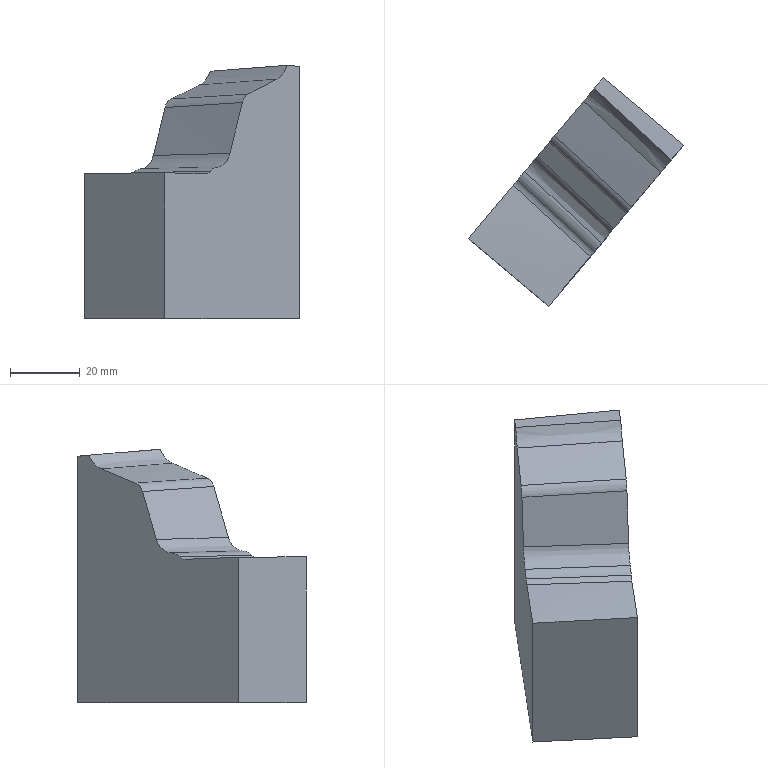Part | NX | features solid 2 | 1 solid | 14 faces | box 61.549 x 65.246 x 72.449 mm | volume 96298 mm3 | spline 9 | plane 5
STEP:
#1=CARTESIAN_POINT('',(566.959,407.194,-45.));
#2=VERTEX_POINT('',#1);
#3=CARTESIAN_POINT('',(566.959,407.194,25.462));
#4=VERTEX_POINT('',#3);
#5=CARTESIAN_POINT('',(566.959,407.194,-5.));
#6=DIRECTION('',(0.,0.,1.));
#7=VECTOR('',#6,1000.);
#8=LINE('',#5,#7);
#9=EDGE_CURVE('',#2,#4,#8,.T.);
#10=ORIENTED_EDGE('',*,*,#9,.T.);
#11=CARTESIAN_POINT('',(589.941,387.91,27.101));
#12=VERTEX_POINT('',#11);
#13=CARTESIAN_POINT('',(566.959,407.194,25.462));
#14=CARTESIAN_POINT('',(574.619,400.767,26.027));
#15=CARTESIAN_POINT('',(582.28,394.339,26.572));
#16=CARTESIAN_POINT('',(589.941,387.91,27.101));
#17=B_SPLINE_CURVE_WITH_KNOTS('',3,(#13,#14,#15,#16),.UNSPECIFIED.,.F.,.F.,(4,4),(0.,0.03004),.UNSPECIFIED.);
#18=EDGE_CURVE('',#4,#12,#17,.T.);
#19=ORIENTED_EDGE('',*,*,#18,.T.);
#20=CARTESIAN_POINT('',(589.941,387.91,-45.));
#21=VERTEX_POINT('',#20);
#22=CARTESIAN_POINT('',(589.941,387.91,-5.));
#23=DIRECTION('',(0.,0.,1.));
#24=VECTOR('',#23,1000.);
#25=LINE('',#22,#24);
#26=EDGE_CURVE('',#21,#12,#25,.T.);
#27=ORIENTED_EDGE('',*,*,#26,.F.);
#28=CARTESIAN_POINT('',(1441.684,-326.787,-45.));
#29=DIRECTION('',(-0.766,0.6428,0.));
#30=VECTOR('',#29,1000.);
#31=LINE('',#28,#30);
#32=EDGE_CURVE('',#2,#21,#31,.F.);
#33=ORIENTED_EDGE('',*,*,#32,.F.);
#34=EDGE_LOOP('',(#10,#19,#27,#33));
#35=FACE_BOUND('',#34,.T.);
#36=CARTESIAN_POINT('',(555.469,416.836,-5.));
#37=DIRECTION('',(0.6428,0.766,0.));
#38=DIRECTION('',(0.,0.,1.));
#39=AXIS2_PLACEMENT_3D('',#36,#37,#38);
#40=PLANE('',#39);
#41=ADVANCED_FACE('',(#35),#40,.T.);
#42=ORIENTED_EDGE('',*,*,#26,.T.);
#43=CARTESIAN_POINT('',(586.365,383.649,27.449));
#44=VERTEX_POINT('',#43);
#45=CARTESIAN_POINT('',(589.941,387.91,27.101));
#46=CARTESIAN_POINT('',(588.749,386.49,27.217));
#47=CARTESIAN_POINT('',(587.557,385.069,27.334));
#48=CARTESIAN_POINT('',(586.365,383.649,27.449));
#49=B_SPLINE_CURVE_WITH_KNOTS('',3,(#45,#46,#47,#48),.UNSPECIFIED.,.F.,.F.,(4,4),(0.,0.005573),.UNSPECIFIED.);
#50=EDGE_CURVE('',#12,#44,#49,.T.);
#51=ORIENTED_EDGE('',*,*,#50,.T.);
#52=CARTESIAN_POINT('',(583.395,380.11,23.455));
#53=VERTEX_POINT('',#52);
#54=CARTESIAN_POINT('',(586.365,383.649,27.449));
#55=CARTESIAN_POINT('',(585.756,382.923,25.561));
#56=CARTESIAN_POINT('',(584.683,381.644,24.119));
#57=CARTESIAN_POINT('',(583.394,380.108,23.454));
#58=B_SPLINE_CURVE_WITH_KNOTS('',3,(#54,#55,#56,#57),.UNSPECIFIED.,.F.,.F.,(4,4),(0.,0.006214),.UNSPECIFIED.);
#59=EDGE_CURVE('',#44,#53,#58,.T.);
#60=ORIENTED_EDGE('',*,*,#59,.T.);
#61=CARTESIAN_POINT('',(575.129,370.258,19.19));
#62=VERTEX_POINT('',#61);
#63=CARTESIAN_POINT('',(583.396,380.111,23.455));
#64=CARTESIAN_POINT('',(580.64,376.826,22.034));
#65=CARTESIAN_POINT('',(577.885,373.542,20.612));
#66=CARTESIAN_POINT('',(575.129,370.258,19.19));
#67=B_SPLINE_CURVE_WITH_KNOTS('',3,(#63,#64,#65,#66),.UNSPECIFIED.,.F.,.F.,(4,4),(0.0002168,0.01377),.UNSPECIFIED.);
#68=EDGE_CURVE('',#53,#62,#67,.T.);
#69=ORIENTED_EDGE('',*,*,#68,.T.);
#70=CARTESIAN_POINT('',(573.535,368.359,16.809));
#71=VERTEX_POINT('',#70);
#72=CARTESIAN_POINT('',(575.129,370.258,19.19));
#73=CARTESIAN_POINT('',(574.4,369.39,18.814));
#74=CARTESIAN_POINT('',(573.806,368.681,17.926));
#75=CARTESIAN_POINT('',(573.535,368.359,16.809));
#76=B_SPLINE_CURVE_WITH_KNOTS('',3,(#72,#73,#74,#75),.UNSPECIFIED.,.F.,.F.,(4,4),(0.,0.003553),.UNSPECIFIED.);
#77=EDGE_CURVE('',#62,#71,#76,.T.);
#78=ORIENTED_EDGE('',*,*,#77,.T.);
#79=CARTESIAN_POINT('',(570.007,364.154,2.246));
#80=VERTEX_POINT('',#79);
#81=CARTESIAN_POINT('',(570.007,364.154,2.246));
#82=CARTESIAN_POINT('',(571.183,365.556,7.1));
#83=CARTESIAN_POINT('',(572.359,366.957,11.954));
#84=CARTESIAN_POINT('',(573.535,368.359,16.809));
#85=B_SPLINE_CURVE_WITH_KNOTS('',3,(#81,#82,#83,#84),.UNSPECIFIED.,.F.,.F.,(4,4),(0.006324,0.02189),.UNSPECIFIED.);
#86=EDGE_CURVE('',#80,#71,#85,.T.);
#87=ORIENTED_EDGE('',*,*,#86,.F.);
#88=CARTESIAN_POINT('',(566.485,359.957,-1.636));
#89=VERTEX_POINT('',#88);
#90=CARTESIAN_POINT('',(570.007,364.154,2.246));
#91=CARTESIAN_POINT('',(569.464,363.507,0.004322));
#92=CARTESIAN_POINT('',(568.025,361.791,-1.579));
#93=CARTESIAN_POINT('',(566.485,359.957,-1.636));
#94=B_SPLINE_CURVE_WITH_KNOTS('',3,(#90,#91,#92,#93),.UNSPECIFIED.,.F.,.F.,(4,4),(0.,0.007083),.UNSPECIFIED.);
#95=EDGE_CURVE('',#80,#89,#94,.T.);
#96=ORIENTED_EDGE('',*,*,#95,.T.);
#97=CARTESIAN_POINT('',(564.485,357.574,-2.817));
#98=VERTEX_POINT('',#97);
#99=CARTESIAN_POINT('',(564.485,357.574,-2.817));
#100=CARTESIAN_POINT('',(565.044,358.239,-2.083));
#101=CARTESIAN_POINT('',(565.755,359.087,-1.664));
#102=CARTESIAN_POINT('',(566.485,359.957,-1.636));
#103=B_SPLINE_CURVE_WITH_KNOTS('',3,(#99,#100,#101,#102),.UNSPECIFIED.,.F.,.F.,(4,4),(0.000003197,0.003403),.UNSPECIFIED.);
#104=EDGE_CURVE('',#98,#89,#103,.T.);
#105=ORIENTED_EDGE('',*,*,#104,.F.);
#106=CARTESIAN_POINT('',(563.201,356.043,-3.525));
#107=VERTEX_POINT('',#106);
#108=CARTESIAN_POINT('',(563.201,356.043,-3.525));
#109=CARTESIAN_POINT('',(563.668,356.6,-3.539));
#110=CARTESIAN_POINT('',(564.129,357.148,-3.285));
#111=CARTESIAN_POINT('',(564.485,357.574,-2.817));
#112=B_SPLINE_CURVE_WITH_KNOTS('',3,(#108,#109,#110,#111),.UNSPECIFIED.,.F.,.F.,(4,4),(0.,0.00217),.UNSPECIFIED.);
#113=EDGE_CURVE('',#107,#98,#112,.T.);
#114=ORIENTED_EDGE('',*,*,#113,.F.);
#115=CARTESIAN_POINT('',(551.374,341.948,-3.282));
#116=VERTEX_POINT('',#115);
#117=CARTESIAN_POINT('',(551.374,341.948,-3.282));
#118=CARTESIAN_POINT('',(555.317,346.647,-3.326));
#119=CARTESIAN_POINT('',(559.259,351.345,-3.407));
#120=CARTESIAN_POINT('',(563.201,356.043,-3.525));
#121=B_SPLINE_CURVE_WITH_KNOTS('',3,(#117,#118,#119,#120),.UNSPECIFIED.,.F.,.F.,(4,4),(0.,0.0184),.UNSPECIFIED.);
#122=EDGE_CURVE('',#116,#107,#121,.T.);
#123=ORIENTED_EDGE('',*,*,#122,.F.);
#124=CARTESIAN_POINT('',(551.374,341.948,-45.));
#125=VERTEX_POINT('',#124);
#126=CARTESIAN_POINT('',(551.374,341.948,-5.));
#127=DIRECTION('',(0.,0.,-1.));
#128=VECTOR('',#127,1000.);
#129=LINE('',#126,#128);
#130=EDGE_CURVE('',#125,#116,#129,.F.);
#131=ORIENTED_EDGE('',*,*,#130,.F.);
#132=CARTESIAN_POINT('',(548.16,338.117,-45.));
#133=DIRECTION('',(-0.6428,-0.766,0.));
#134=VECTOR('',#133,1000.);
#135=LINE('',#132,#134);
#136=EDGE_CURVE('',#125,#21,#135,.F.);
#137=ORIENTED_EDGE('',*,*,#136,.T.);
#138=EDGE_LOOP('',(#42,#51,#60,#69,#78,#87,#96,#105,#114,#123,#131,#137));
#139=FACE_BOUND('',#138,.T.);
#140=CARTESIAN_POINT('',(548.16,338.117,-5.));
#141=DIRECTION('',(0.766,-0.6428,0.));
#142=DIRECTION('',(0.6428,0.766,0.));
#143=AXIS2_PLACEMENT_3D('',#140,#141,#142);
#144=PLANE('',#143);
#145=ADVANCED_FACE('',(#139),#144,.T.);
#146=CARTESIAN_POINT('',(564.326,404.056,25.737));
#147=VERTEX_POINT('',#146);
#148=CARTESIAN_POINT('',(566.959,407.194,25.462));
#149=CARTESIAN_POINT('',(566.082,406.148,25.554));
#150=CARTESIAN_POINT('',(565.204,405.102,25.646));
#151=CARTESIAN_POINT('',(564.326,404.056,25.737));
#152=B_SPLINE_CURVE_WITH_KNOTS('',3,(#148,#149,#150,#151),.UNSPECIFIED.,.F.,.F.,(4,4),(0.,0.004106),.UNSPECIFIED.);
#153=EDGE_CURVE('',#4,#147,#152,.T.);
#154=ORIENTED_EDGE('',*,*,#153,.F.);
#155=ORIENTED_EDGE('',*,*,#9,.F.);
#156=CARTESIAN_POINT('',(528.392,361.231,-45.));
#157=VERTEX_POINT('',#156);
#158=CARTESIAN_POINT('',(525.178,357.401,-45.));
#159=DIRECTION('',(-0.6428,-0.766,0.));
#160=VECTOR('',#159,1000.);
#161=LINE('',#158,#160);
#162=EDGE_CURVE('',#157,#2,#161,.F.);
#163=ORIENTED_EDGE('',*,*,#162,.F.);
#164=CARTESIAN_POINT('',(528.392,361.231,-3.433));
#165=VERTEX_POINT('',#164);
#166=CARTESIAN_POINT('',(528.392,361.231,-5.));
#167=DIRECTION('',(0.,0.,-1.));
#168=VECTOR('',#167,1000.);
#169=LINE('',#166,#168);
#170=EDGE_CURVE('',#157,#165,#169,.F.);
#171=ORIENTED_EDGE('',*,*,#170,.T.);
#172=CARTESIAN_POINT('',(541.163,376.451,-3.994));
#173=VERTEX_POINT('',#172);
#174=CARTESIAN_POINT('',(528.392,361.231,-3.433));
#175=CARTESIAN_POINT('',(532.65,366.305,-3.577));
#176=CARTESIAN_POINT('',(536.907,371.379,-3.764));
#177=CARTESIAN_POINT('',(541.163,376.451,-3.994));
#178=B_SPLINE_CURVE_WITH_KNOTS('',3,(#174,#175,#176,#177),.UNSPECIFIED.,.F.,.F.,(4,4),(0.,0.01988),.UNSPECIFIED.);
#179=EDGE_CURVE('',#165,#173,#178,.T.);
#180=ORIENTED_EDGE('',*,*,#179,.T.);
#181=CARTESIAN_POINT('',(542.453,377.988,-3.316));
#182=VERTEX_POINT('',#181);
#183=CARTESIAN_POINT('',(541.163,376.451,-3.994));
#184=CARTESIAN_POINT('',(541.63,377.007,-4.019));
#185=CARTESIAN_POINT('',(542.092,377.558,-3.777));
#186=CARTESIAN_POINT('',(542.453,377.988,-3.316));
#187=B_SPLINE_CURVE_WITH_KNOTS('',3,(#183,#184,#185,#186),.UNSPECIFIED.,.F.,.F.,(4,4),(0.,0.002169),.UNSPECIFIED.);
#188=EDGE_CURVE('',#173,#182,#187,.T.);
#189=ORIENTED_EDGE('',*,*,#188,.T.);
#190=CARTESIAN_POINT('',(544.495,380.422,-2.184));
#191=VERTEX_POINT('',#190);
#192=CARTESIAN_POINT('',(542.453,377.988,-3.316));
#193=CARTESIAN_POINT('',(543.027,378.672,-2.585));
#194=CARTESIAN_POINT('',(543.754,379.539,-2.182));
#195=CARTESIAN_POINT('',(544.495,380.422,-2.184));
#196=B_SPLINE_CURVE_WITH_KNOTS('',3,(#192,#193,#194,#195),.UNSPECIFIED.,.F.,.F.,(4,4),(0.000003374,0.003451),.UNSPECIFIED.);
#197=EDGE_CURVE('',#182,#191,#196,.T.);
#198=ORIENTED_EDGE('',*,*,#197,.T.);
#199=CARTESIAN_POINT('',(548.104,384.723,1.672));
#200=VERTEX_POINT('',#199);
#201=CARTESIAN_POINT('',(548.104,384.723,1.672));
#202=CARTESIAN_POINT('',(547.546,384.058,-0.6026));
#203=CARTESIAN_POINT('',(546.061,382.288,-2.188));
#204=CARTESIAN_POINT('',(544.495,380.422,-2.184));
#205=B_SPLINE_CURVE_WITH_KNOTS('',3,(#201,#202,#203,#204),.UNSPECIFIED.,.F.,.F.,(4,4),(0.,0.007202),.UNSPECIFIED.);
#206=EDGE_CURVE('',#200,#191,#205,.T.);
#207=ORIENTED_EDGE('',*,*,#206,.F.);
#208=CARTESIAN_POINT('',(551.467,388.73,15.371));
#209=VERTEX_POINT('',#208);
#210=CARTESIAN_POINT('',(548.104,384.723,1.672));
#211=CARTESIAN_POINT('',(549.225,386.059,6.238));
#212=CARTESIAN_POINT('',(550.346,387.395,10.805));
#213=CARTESIAN_POINT('',(551.467,388.73,15.371));
#214=B_SPLINE_CURVE_WITH_KNOTS('',3,(#210,#211,#212,#213),.UNSPECIFIED.,.F.,.F.,(4,4),(0.006972,0.02164),.UNSPECIFIED.);
#215=EDGE_CURVE('',#200,#209,#214,.T.);
#216=ORIENTED_EDGE('',*,*,#215,.T.);
#217=CARTESIAN_POINT('',(553.09,390.665,17.754));
#218=VERTEX_POINT('',#217);
#219=CARTESIAN_POINT('',(553.09,390.665,17.754));
#220=CARTESIAN_POINT('',(552.35,389.783,17.39));
#221=CARTESIAN_POINT('',(551.743,389.06,16.499));
#222=CARTESIAN_POINT('',(551.467,388.73,15.371));
#223=B_SPLINE_CURVE_WITH_KNOTS('',3,(#219,#220,#221,#222),.UNSPECIFIED.,.F.,.F.,(4,4),(0.,0.003592),.UNSPECIFIED.);
#224=EDGE_CURVE('',#218,#209,#223,.T.);
#225=ORIENTED_EDGE('',*,*,#224,.F.);
#226=CARTESIAN_POINT('',(561.322,400.475,21.808));
#227=VERTEX_POINT('',#226);
#228=CARTESIAN_POINT('',(561.323,400.476,21.808));
#229=CARTESIAN_POINT('',(558.578,397.206,20.457));
#230=CARTESIAN_POINT('',(555.834,393.935,19.106));
#231=CARTESIAN_POINT('',(553.09,390.665,17.754));
#232=B_SPLINE_CURVE_WITH_KNOTS('',3,(#228,#229,#230,#231),.UNSPECIFIED.,.F.,.F.,(4,4),(0.0001803,0.01361),.UNSPECIFIED.);
#233=EDGE_CURVE('',#227,#218,#232,.T.);
#234=ORIENTED_EDGE('',*,*,#233,.F.);
#235=CARTESIAN_POINT('',(564.326,404.056,25.737));
#236=CARTESIAN_POINT('',(563.7,403.31,23.864));
#237=CARTESIAN_POINT('',(562.615,402.017,22.445));
#238=CARTESIAN_POINT('',(561.322,400.475,21.808));
#239=B_SPLINE_CURVE_WITH_KNOTS('',3,(#235,#236,#237,#238),.UNSPECIFIED.,.F.,.F.,(4,4),(0.,0.006211),.UNSPECIFIED.);
#240=EDGE_CURVE('',#147,#227,#239,.T.);
#241=ORIENTED_EDGE('',*,*,#240,.F.);
#242=EDGE_LOOP('',(#154,#155,#163,#171,#180,#189,#198,#207,#216,#225,#234,#241));
#243=FACE_BOUND('',#242,.T.);
#244=CARTESIAN_POINT('',(525.178,357.401,-5.));
#245=DIRECTION('',(0.766,-0.6428,0.));
#246=DIRECTION('',(0.6428,0.766,0.));
#247=AXIS2_PLACEMENT_3D('',#244,#245,#246);
#248=PLANE('',#247);
#249=ADVANCED_FACE('',(#243),#248,.F.);
#250=ORIENTED_EDGE('',*,*,#130,.T.);
#251=CARTESIAN_POINT('',(528.392,361.231,-3.433));
#252=CARTESIAN_POINT('',(536.052,354.803,-3.328));
#253=CARTESIAN_POINT('',(543.713,348.376,-3.277));
#254=CARTESIAN_POINT('',(551.374,341.948,-3.282));
#255=B_SPLINE_CURVE_WITH_KNOTS('',3,(#251,#252,#253,#254),.UNSPECIFIED.,.F.,.F.,(4,4),(0.,0.03),.UNSPECIFIED.);
#256=EDGE_CURVE('',#165,#116,#255,.T.);
#257=ORIENTED_EDGE('',*,*,#256,.F.);
#258=ORIENTED_EDGE('',*,*,#170,.F.);
#259=CARTESIAN_POINT('',(516.902,370.873,-45.));
#260=DIRECTION('',(0.766,-0.6428,0.));
#261=VECTOR('',#260,1000.);
#262=LINE('',#259,#261);
#263=EDGE_CURVE('',#157,#125,#262,.T.);
#264=ORIENTED_EDGE('',*,*,#263,.T.);
#265=EDGE_LOOP('',(#250,#257,#258,#264));
#266=FACE_BOUND('',#265,.T.);
#267=CARTESIAN_POINT('',(516.902,370.873,-5.));
#268=DIRECTION('',(0.6428,0.766,0.));
#269=DIRECTION('',(0.,0.,1.));
#270=AXIS2_PLACEMENT_3D('',#267,#268,#269);
#271=PLANE('',#270);
#272=ADVANCED_FACE('',(#266),#271,.F.);
#273=ORIENTED_EDGE('',*,*,#263,.F.);
#274=ORIENTED_EDGE('',*,*,#162,.T.);
#275=ORIENTED_EDGE('',*,*,#32,.T.);
#276=ORIENTED_EDGE('',*,*,#136,.F.);
#277=EDGE_LOOP('',(#273,#274,#275,#276));
#278=FACE_BOUND('',#277,.T.);
#279=CARTESIAN_POINT('',(1076.581,-761.9,-45.));
#280=DIRECTION('',(0.,0.,1.));
#281=DIRECTION('',(1.,0.,0.));
#282=AXIS2_PLACEMENT_3D('',#279,#280,#281);
#283=PLANE('',#282);
#284=ADVANCED_FACE('',(#278),#283,.F.);
#285=CARTESIAN_POINT('',(541.163,376.451,-3.994));
#286=CARTESIAN_POINT('',(548.532,369.705,-3.778));
#287=CARTESIAN_POINT('',(555.864,362.916,-3.62));
#288=CARTESIAN_POINT('',(563.201,356.043,-3.525));
#289=B_SPLINE_CURVE_WITH_KNOTS('',3,(#285,#286,#287,#288),.UNSPECIFIED.,.F.,.F.,(4,4),(0.5481,0.8366),.UNSPECIFIED.);
#290=EDGE_CURVE('',#173,#107,#289,.T.);
#291=ORIENTED_EDGE('',*,*,#290,.T.);
#292=ORIENTED_EDGE('',*,*,#113,.T.);
#293=CARTESIAN_POINT('',(564.485,357.574,-2.817));
#294=CARTESIAN_POINT('',(557.239,364.365,-2.921));
#295=CARTESIAN_POINT('',(549.881,371.184,-3.088));
#296=CARTESIAN_POINT('',(542.453,377.988,-3.316));
#297=B_SPLINE_CURVE_WITH_KNOTS('',3,(#293,#294,#295,#296),.UNSPECIFIED.,.F.,.F.,(4,4),(0.1708,0.4613),.UNSPECIFIED.);
#298=EDGE_CURVE('',#98,#182,#297,.T.);
#299=ORIENTED_EDGE('',*,*,#298,.T.);
#300=ORIENTED_EDGE('',*,*,#188,.F.);
#301=EDGE_LOOP('',(#291,#292,#299,#300));
#302=FACE_BOUND('',#301,.T.);
#303=CARTESIAN_POINT('',(540.974,376.624,-4.));
#304=CARTESIAN_POINT('',(541.267,376.942,-4.014));
#305=CARTESIAN_POINT('',(541.56,377.264,-3.951));
#306=CARTESIAN_POINT('',(541.841,377.575,-3.809));
#307=CARTESIAN_POINT('',(542.097,377.861,-3.595));
#308=CARTESIAN_POINT('',(542.319,378.111,-3.321));
#309=CARTESIAN_POINT('',(541.45,376.188,-3.986));
#310=CARTESIAN_POINT('',(541.743,376.506,-4.));
#311=CARTESIAN_POINT('',(542.036,376.828,-3.937));
#312=CARTESIAN_POINT('',(542.317,377.138,-3.795));
#313=CARTESIAN_POINT('',(542.574,377.424,-3.58));
#314=CARTESIAN_POINT('',(542.795,377.675,-3.306));
#315=CARTESIAN_POINT('',(541.926,375.752,-3.972));
#316=CARTESIAN_POINT('',(542.219,376.07,-3.986));
#317=CARTESIAN_POINT('',(542.513,376.392,-3.923));
#318=CARTESIAN_POINT('',(542.794,376.702,-3.781));
#319=CARTESIAN_POINT('',(543.05,376.988,-3.566));
#320=CARTESIAN_POINT('',(543.272,377.238,-3.291));
#321=CARTESIAN_POINT('',(542.403,375.316,-3.958));
#322=CARTESIAN_POINT('',(542.696,375.634,-3.973));
#323=CARTESIAN_POINT('',(542.989,375.955,-3.909));
#324=CARTESIAN_POINT('',(543.27,376.265,-3.766));
#325=CARTESIAN_POINT('',(543.527,376.551,-3.552));
#326=CARTESIAN_POINT('',(543.749,376.801,-3.277));
#327=CARTESIAN_POINT('',(545.037,372.9,-3.884));
#328=CARTESIAN_POINT('',(545.33,373.218,-3.898));
#329=CARTESIAN_POINT('',(545.624,373.539,-3.833));
#330=CARTESIAN_POINT('',(545.906,373.849,-3.69));
#331=CARTESIAN_POINT('',(546.162,374.133,-3.475));
#332=CARTESIAN_POINT('',(546.385,374.382,-3.199));
#333=CARTESIAN_POINT('',(547.66,370.487,-3.816));
#334=CARTESIAN_POINT('',(547.954,370.804,-3.829));
#335=CARTESIAN_POINT('',(548.248,371.124,-3.764));
#336=CARTESIAN_POINT('',(548.53,371.433,-3.62));
#337=CARTESIAN_POINT('',(548.787,371.717,-3.404));
#338=CARTESIAN_POINT('',(549.01,371.965,-3.128));
#339=CARTESIAN_POINT('',(549.8,368.512,-3.765));
#340=CARTESIAN_POINT('',(550.094,368.83,-3.777));
#341=CARTESIAN_POINT('',(550.388,369.149,-3.711));
#342=CARTESIAN_POINT('',(550.671,369.458,-3.567));
#343=CARTESIAN_POINT('',(550.928,369.741,-3.35));
#344=CARTESIAN_POINT('',(551.151,369.988,-3.074));
#345=CARTESIAN_POINT('',(552.884,365.659,-3.698));
#346=CARTESIAN_POINT('',(553.178,365.976,-3.709));
#347=CARTESIAN_POINT('',(553.473,366.295,-3.642));
#348=CARTESIAN_POINT('',(553.756,366.603,-3.497));
#349=CARTESIAN_POINT('',(554.014,366.885,-3.279));
#350=CARTESIAN_POINT('',(554.237,367.131,-3.002));
#351=CARTESIAN_POINT('',(555.953,362.809,-3.639));
#352=CARTESIAN_POINT('',(556.248,363.125,-3.65));
#353=CARTESIAN_POINT('',(556.543,363.443,-3.582));
#354=CARTESIAN_POINT('',(556.826,363.75,-3.436));
#355=CARTESIAN_POINT('',(557.085,364.031,-3.217));
#356=CARTESIAN_POINT('',(557.308,364.276,-2.939));
#357=CARTESIAN_POINT('',(556.896,361.931,-3.622));
#358=CARTESIAN_POINT('',(557.191,362.248,-3.632));
#359=CARTESIAN_POINT('',(557.486,362.566,-3.564));
#360=CARTESIAN_POINT('',(557.77,362.872,-3.418));
#361=CARTESIAN_POINT('',(558.028,363.153,-3.199));
#362=CARTESIAN_POINT('',(558.252,363.398,-2.921));
#363=CARTESIAN_POINT('',(558.752,360.203,-3.59));
#364=CARTESIAN_POINT('',(559.048,360.519,-3.599));
#365=CARTESIAN_POINT('',(559.344,360.836,-3.531));
#366=CARTESIAN_POINT('',(559.627,361.142,-3.384));
#367=CARTESIAN_POINT('',(559.886,361.423,-3.165));
#368=CARTESIAN_POINT('',(560.109,361.667,-2.886));
#369=CARTESIAN_POINT('',(560.603,358.475,-3.561));
#370=CARTESIAN_POINT('',(560.899,358.79,-3.57));
#371=CARTESIAN_POINT('',(561.195,359.108,-3.501));
#372=CARTESIAN_POINT('',(561.479,359.413,-3.353));
#373=CARTESIAN_POINT('',(561.738,359.693,-3.134));
#374=CARTESIAN_POINT('',(561.962,359.936,-2.855));
#375=CARTESIAN_POINT('',(561.514,357.623,-3.548));
#376=CARTESIAN_POINT('',(561.81,357.939,-3.557));
#377=CARTESIAN_POINT('',(562.107,358.256,-3.487));
#378=CARTESIAN_POINT('',(562.391,358.561,-3.339));
#379=CARTESIAN_POINT('',(562.65,358.84,-3.12));
#380=CARTESIAN_POINT('',(562.874,359.084,-2.84));
#381=CARTESIAN_POINT('',(562.424,356.772,-3.535));
#382=CARTESIAN_POINT('',(562.72,357.087,-3.544));
#383=CARTESIAN_POINT('',(563.017,357.404,-3.474));
#384=CARTESIAN_POINT('',(563.301,357.709,-3.326));
#385=CARTESIAN_POINT('',(563.56,357.988,-3.106));
#386=CARTESIAN_POINT('',(563.784,358.231,-2.827));
#387=CARTESIAN_POINT('',(563.332,355.921,-3.524));
#388=CARTESIAN_POINT('',(563.629,356.236,-3.532));
#389=CARTESIAN_POINT('',(563.925,356.553,-3.462));
#390=CARTESIAN_POINT('',(564.21,356.858,-3.313));
#391=CARTESIAN_POINT('',(564.469,357.136,-3.093));
#392=CARTESIAN_POINT('',(564.693,357.379,-2.814));
#393=B_SPLINE_SURFACE_WITH_KNOTS('',5,5,((#303,#304,#305,#306,#307,#308),(#309,#310,#311,#312,#313,#314),(#315,#316,#317,#318,#319,#320),(#321,#322,#323,#324,#325,#326),(#327,#328,#329,#330,#331,#332),(#333,#334,#335,#336,#337,#338),(#339,#340,#341,#342,#343,#344),(#345,#346,#347,#348,#349,#350),(#351,#352,#353,#354,#355,#356),(#357,#358,#359,#360,#361,#362),(#363,#364,#365,#366,#367,#368),(#369,#370,#371,#372,#373,#374),(#375,#376,#377,#378,#379,#380),(#381,#382,#383,#384,#385,#386),(#387,#388,#389,#390,#391,#392)),.UNSPECIFIED.,.F.,.F.,.F.,(6,3,3,3,6),(6,6),(0.537,0.568,0.7087,0.7712,0.832),(0.,1.),.UNSPECIFIED.);
#394=ADVANCED_FACE('',(#302),#393,.T.);
#395=ORIENTED_EDGE('',*,*,#298,.F.);
#396=ORIENTED_EDGE('',*,*,#104,.T.);
#397=CARTESIAN_POINT('',(566.485,359.957,-1.636));
#398=CARTESIAN_POINT('',(564.733,361.609,-1.666));
#399=CARTESIAN_POINT('',(562.019,364.16,-1.716));
#400=CARTESIAN_POINT('',(558.279,367.657,-1.798));
#401=CARTESIAN_POINT('',(556.002,369.779,-1.852));
#402=CARTESIAN_POINT('',(554.201,371.454,-1.898));
#403=CARTESIAN_POINT('',(552.911,372.652,-1.932));
#404=CARTESIAN_POINT('',(551.301,374.145,-1.976));
#405=CARTESIAN_POINT('',(549.875,375.465,-2.017));
#406=CARTESIAN_POINT('',(548.553,376.686,-2.056));
#407=CARTESIAN_POINT('',(546.747,378.351,-2.111));
#408=CARTESIAN_POINT('',(545.398,379.593,-2.154));
#409=CARTESIAN_POINT('',(544.495,380.422,-2.184));
#410=B_SPLINE_CURVE_WITH_KNOTS('',3,(#397,#398,#399,#400,#401,#402,#403,#404,#405,#406,#407,#408,#409),.UNSPECIFIED.,.F.,.F.,(4,1,1,1,1,1,1,1,1,1,4),(0.1737,0.2446,0.2801,0.3156,0.3334,0.3511,0.3689,0.3866,0.4044,0.4221,0.4576),.UNSPECIFIED.);
#411=EDGE_CURVE('',#89,#191,#410,.T.);
#412=ORIENTED_EDGE('',*,*,#411,.T.);
#413=ORIENTED_EDGE('',*,*,#197,.F.);
#414=EDGE_LOOP('',(#395,#396,#412,#413));
#415=FACE_BOUND('',#414,.T.);
#416=CARTESIAN_POINT('',(566.77,359.779,-1.631));
#417=CARTESIAN_POINT('',(566.299,359.273,-1.639));
#418=CARTESIAN_POINT('',(565.829,358.768,-1.767));
#419=CARTESIAN_POINT('',(565.38,358.283,-2.014));
#420=CARTESIAN_POINT('',(564.971,357.838,-2.37));
#421=CARTESIAN_POINT('',(564.615,357.449,-2.817));
#422=CARTESIAN_POINT('',(565.115,361.333,-1.659));
#423=CARTESIAN_POINT('',(564.643,360.827,-1.666));
#424=CARTESIAN_POINT('',(564.174,360.321,-1.793));
#425=CARTESIAN_POINT('',(563.725,359.835,-2.039));
#426=CARTESIAN_POINT('',(563.316,359.39,-2.394));
#427=CARTESIAN_POINT('',(562.961,358.999,-2.841));
#428=CARTESIAN_POINT('',(563.454,362.887,-1.689));
#429=CARTESIAN_POINT('',(562.984,362.381,-1.695));
#430=CARTESIAN_POINT('',(562.515,361.875,-1.821));
#431=CARTESIAN_POINT('',(562.067,361.388,-2.067));
#432=CARTESIAN_POINT('',(561.658,360.942,-2.421));
#433=CARTESIAN_POINT('',(561.302,360.551,-2.867));
#434=CARTESIAN_POINT('',(561.79,364.442,-1.721));
#435=CARTESIAN_POINT('',(561.32,363.936,-1.727));
#436=CARTESIAN_POINT('',(560.851,363.429,-1.852));
#437=CARTESIAN_POINT('',(560.404,362.942,-2.097));
#438=CARTESIAN_POINT('',(559.995,362.494,-2.451));
#439=CARTESIAN_POINT('',(559.64,362.102,-2.896));
#440=CARTESIAN_POINT('',(557.337,368.595,-1.816));
#441=CARTESIAN_POINT('',(556.868,368.087,-1.82));
#442=CARTESIAN_POINT('',(556.4,367.579,-1.943));
#443=CARTESIAN_POINT('',(555.954,367.089,-2.185));
#444=CARTESIAN_POINT('',(555.546,366.639,-2.537));
#445=CARTESIAN_POINT('',(555.192,366.245,-2.981));
#446=CARTESIAN_POINT('',(552.853,372.751,-1.93));
#447=CARTESIAN_POINT('',(552.385,372.242,-1.931));
#448=CARTESIAN_POINT('',(551.919,371.732,-2.052));
#449=CARTESIAN_POINT('',(551.473,371.241,-2.293));
#450=CARTESIAN_POINT('',(551.066,370.789,-2.643));
#451=CARTESIAN_POINT('',(550.713,370.392,-3.085));
#452=CARTESIAN_POINT('',(550.038,375.351,-2.008));
#453=CARTESIAN_POINT('',(549.571,374.842,-2.009));
#454=CARTESIAN_POINT('',(549.105,374.331,-2.128));
#455=CARTESIAN_POINT('',(548.66,373.838,-2.368));
#456=CARTESIAN_POINT('',(548.254,373.385,-2.717));
#457=CARTESIAN_POINT('',(547.901,372.986,-3.158));
#458=CARTESIAN_POINT('',(547.211,377.953,-2.095));
#459=CARTESIAN_POINT('',(546.744,377.443,-2.094));
#460=CARTESIAN_POINT('',(546.279,376.931,-2.212));
#461=CARTESIAN_POINT('',(545.835,376.437,-2.45));
#462=CARTESIAN_POINT('',(545.429,375.982,-2.798));
#463=CARTESIAN_POINT('',(545.076,375.582,-3.238));
#464=CARTESIAN_POINT('',(544.371,380.557,-2.189));
#465=CARTESIAN_POINT('',(543.905,380.046,-2.186));
#466=CARTESIAN_POINT('',(543.441,379.533,-2.303));
#467=CARTESIAN_POINT('',(542.997,379.038,-2.54));
#468=CARTESIAN_POINT('',(542.592,378.582,-2.886));
#469=CARTESIAN_POINT('',(542.24,378.18,-3.325));
#470=B_SPLINE_SURFACE_WITH_KNOTS('',5,5,((#416,#417,#418,#419,#420,#421),(#422,#423,#424,#425,#426,#427),(#428,#429,#430,#431,#432,#433),(#434,#435,#436,#437,#438,#439),(#440,#441,#442,#443,#444,#445),(#446,#447,#448,#449,#450,#451),(#452,#453,#454,#455,#456,#457),(#458,#459,#460,#461,#462,#463),(#464,#465,#466,#467,#468,#469)),.UNSPECIFIED.,.F.,.F.,.F.,(6,3,6),(6,6),(0.1683,0.2783,0.4618),(0.,1.),.UNSPECIFIED.);
#471=ADVANCED_FACE('',(#415),#470,.T.);
#472=ORIENTED_EDGE('',*,*,#206,.T.);
#473=ORIENTED_EDGE('',*,*,#411,.F.);
#474=ORIENTED_EDGE('',*,*,#95,.F.);
#475=CARTESIAN_POINT('',(548.104,384.723,1.672));
#476=CARTESIAN_POINT('',(555.53,377.849,1.927));
#477=CARTESIAN_POINT('',(562.819,371.001,2.118));
#478=CARTESIAN_POINT('',(570.007,364.154,2.246));
#479=B_SPLINE_CURVE_WITH_KNOTS('',3,(#475,#476,#477,#478),.UNSPECIFIED.,.F.,.F.,(4,4),(0.5365,0.8266),.UNSPECIFIED.);
#480=EDGE_CURVE('',#200,#80,#479,.T.);
#481=ORIENTED_EDGE('',*,*,#480,.F.);
#482=EDGE_LOOP('',(#472,#473,#474,#481));
#483=FACE_BOUND('',#482,.T.);
#484=CARTESIAN_POINT('',(566.616,359.834,-1.634));
#485=CARTESIAN_POINT('',(567.598,360.864,-1.599));
#486=CARTESIAN_POINT('',(568.569,361.89,-1.141));
#487=CARTESIAN_POINT('',(569.413,362.79,-0.2641));
#488=CARTESIAN_POINT('',(570.021,363.448,0.9195));
#489=CARTESIAN_POINT('',(570.356,363.821,2.252));
#490=CARTESIAN_POINT('',(566.277,360.154,-1.64));
#491=CARTESIAN_POINT('',(567.259,361.185,-1.605));
#492=CARTESIAN_POINT('',(568.23,362.211,-1.148));
#493=CARTESIAN_POINT('',(569.074,363.112,-0.2707));
#494=CARTESIAN_POINT('',(569.682,363.771,0.9132));
#495=CARTESIAN_POINT('',(570.016,364.145,2.246));
#496=CARTESIAN_POINT('',(565.937,360.474,-1.646));
#497=CARTESIAN_POINT('',(566.919,361.505,-1.611));
#498=CARTESIAN_POINT('',(567.89,362.533,-1.155));
#499=CARTESIAN_POINT('',(568.734,363.434,-0.2774));
#500=CARTESIAN_POINT('',(569.343,364.094,0.9067));
#501=CARTESIAN_POINT('',(569.677,364.468,2.24));
#502=CARTESIAN_POINT('',(565.597,360.794,-1.651));
#503=CARTESIAN_POINT('',(566.579,361.826,-1.618));
#504=CARTESIAN_POINT('',(567.55,362.854,-1.161));
#505=CARTESIAN_POINT('',(568.395,363.757,-0.2843));
#506=CARTESIAN_POINT('',(569.003,364.417,0.9002));
#507=CARTESIAN_POINT('',(569.337,364.791,2.234));
#508=CARTESIAN_POINT('',(564.816,361.53,-1.665));
#509=CARTESIAN_POINT('',(565.798,362.563,-1.633));
#510=CARTESIAN_POINT('',(566.77,363.593,-1.177));
#511=CARTESIAN_POINT('',(567.614,364.497,-0.3002));
#512=CARTESIAN_POINT('',(568.223,365.159,0.8848));
#513=CARTESIAN_POINT('',(568.557,365.534,2.219));
#514=CARTESIAN_POINT('',(564.033,362.266,-1.679));
#515=CARTESIAN_POINT('',(565.016,363.3,-1.649));
#516=CARTESIAN_POINT('',(565.988,364.331,-1.194));
#517=CARTESIAN_POINT('',(566.833,365.237,-0.3168));
#518=CARTESIAN_POINT('',(567.441,365.9,0.8689));
#519=CARTESIAN_POINT('',(567.775,366.277,2.204));
#520=CARTESIAN_POINT('',(563.591,362.681,-1.688));
#521=CARTESIAN_POINT('',(564.574,363.716,-1.658));
#522=CARTESIAN_POINT('',(565.546,364.748,-1.203));
#523=CARTESIAN_POINT('',(566.391,365.655,-0.3263));
#524=CARTESIAN_POINT('',(567.,366.319,0.8597));
#525=CARTESIAN_POINT('',(567.333,366.697,2.195));
#526=CARTESIAN_POINT('',(561.036,365.081,-1.736));
#527=CARTESIAN_POINT('',(562.019,366.12,-1.711));
#528=CARTESIAN_POINT('',(562.992,367.157,-1.259));
#529=CARTESIAN_POINT('',(563.838,368.07,-0.3824));
#530=CARTESIAN_POINT('',(564.447,368.739,0.8054));
#531=CARTESIAN_POINT('',(564.78,369.12,2.144));
#532=CARTESIAN_POINT('',(558.471,367.481,-1.792));
#533=CARTESIAN_POINT('',(559.454,368.524,-1.771));
#534=CARTESIAN_POINT('',(560.428,369.567,-1.322));
#535=CARTESIAN_POINT('',(561.275,370.485,-0.4448));
#536=CARTESIAN_POINT('',(561.884,371.159,0.7448));
#537=CARTESIAN_POINT('',(562.216,371.543,2.086));
#538=CARTESIAN_POINT('',(556.342,369.466,-1.842));
#539=CARTESIAN_POINT('',(557.326,370.512,-1.824));
#540=CARTESIAN_POINT('',(558.301,371.559,-1.377));
#541=CARTESIAN_POINT('',(559.148,372.482,-0.5006));
#542=CARTESIAN_POINT('',(559.757,373.16,0.6902));
#543=CARTESIAN_POINT('',(560.088,373.546,2.033));
#544=CARTESIAN_POINT('',(552.658,372.891,-1.936));
#545=CARTESIAN_POINT('',(553.643,373.943,-1.924));
#546=CARTESIAN_POINT('',(554.618,374.997,-1.481));
#547=CARTESIAN_POINT('',(555.466,375.928,-0.6044));
#548=CARTESIAN_POINT('',(556.074,376.612,0.5886));
#549=CARTESIAN_POINT('',(556.404,377.003,1.935));
#550=CARTESIAN_POINT('',(548.953,376.318,-2.043));
#551=CARTESIAN_POINT('',(549.938,377.374,-2.037));
#552=CARTESIAN_POINT('',(550.914,378.436,-1.597));
#553=CARTESIAN_POINT('',(551.762,379.374,-0.7209));
#554=CARTESIAN_POINT('',(552.37,380.065,0.4741));
#555=CARTESIAN_POINT('',(552.698,380.46,1.823));
#556=CARTESIAN_POINT('',(547.377,377.772,-2.091));
#557=CARTESIAN_POINT('',(548.362,378.83,-2.087));
#558=CARTESIAN_POINT('',(549.338,379.895,-1.648));
#559=CARTESIAN_POINT('',(550.186,380.836,-0.7726));
#560=CARTESIAN_POINT('',(550.794,381.529,0.4232));
#561=CARTESIAN_POINT('',(551.121,381.927,1.774));
#562=CARTESIAN_POINT('',(545.8,379.224,-2.141));
#563=CARTESIAN_POINT('',(546.784,380.284,-2.139));
#564=CARTESIAN_POINT('',(547.761,381.352,-1.702));
#565=CARTESIAN_POINT('',(548.609,382.296,-0.8265));
#566=CARTESIAN_POINT('',(549.216,382.992,0.37));
#567=CARTESIAN_POINT('',(549.544,383.391,1.722));
#568=CARTESIAN_POINT('',(544.224,380.671,-2.193));
#569=CARTESIAN_POINT('',(545.209,381.734,-2.194));
#570=CARTESIAN_POINT('',(546.185,382.804,-1.758));
#571=CARTESIAN_POINT('',(547.034,383.751,-0.8824));
#572=CARTESIAN_POINT('',(547.64,384.449,0.3147));
#573=CARTESIAN_POINT('',(547.967,384.851,1.668));
#574=B_SPLINE_SURFACE_WITH_KNOTS('',5,5,((#484,#485,#486,#487,#488,#489),(#490,#491,#492,#493,#494,#495),(#496,#497,#498,#499,#500,#501),(#502,#503,#504,#505,#506,#507),(#508,#509,#510,#511,#512,#513),(#514,#515,#516,#517,#518,#519),(#520,#521,#522,#523,#524,#525),(#526,#527,#528,#529,#530,#531),(#532,#533,#534,#535,#536,#537),(#538,#539,#540,#541,#542,#543),(#544,#545,#546,#547,#548,#549),(#550,#551,#552,#553,#554,#555),(#556,#557,#558,#559,#560,#561),(#562,#563,#564,#565,#566,#567),(#568,#569,#570,#571,#572,#573)),.UNSPECIFIED.,.F.,.F.,.F.,(6,3,3,3,6),(6,6),(0.1687,0.1915,0.2211,0.3626,0.4653),(0.,1.),.UNSPECIFIED.);
#575=ADVANCED_FACE('',(#483),#574,.F.);
#576=ORIENTED_EDGE('',*,*,#480,.T.);
#577=ORIENTED_EDGE('',*,*,#86,.T.);
#578=CARTESIAN_POINT('',(573.535,368.359,16.809));
#579=CARTESIAN_POINT('',(569.804,371.843,16.575));
#580=CARTESIAN_POINT('',(562.506,378.617,16.108));
#581=CARTESIAN_POINT('',(555.151,385.368,15.62));
#582=CARTESIAN_POINT('',(551.467,388.73,15.371));
#583=B_SPLINE_CURVE_WITH_KNOTS('',3,(#578,#579,#580,#581,#582),.UNSPECIFIED.,.F.,.F.,(4,1,4),(0.2733,0.3375,0.4017),.UNSPECIFIED.);
#584=EDGE_CURVE('',#71,#209,#583,.T.);
#585=ORIENTED_EDGE('',*,*,#584,.T.);
#586=ORIENTED_EDGE('',*,*,#215,.F.);
#587=EDGE_LOOP('',(#576,#577,#585,#586));
#588=FACE_BOUND('',#587,.T.);
#589=CARTESIAN_POINT('',(547.815,384.63,0.9737));
#590=CARTESIAN_POINT('',(551.117,389.22,15.672));
#591=CARTESIAN_POINT('',(552.344,380.488,1.225));
#592=CARTESIAN_POINT('',(555.654,385.054,15.929));
#593=CARTESIAN_POINT('',(556.862,376.334,1.47));
#594=CARTESIAN_POINT('',(560.18,380.875,16.18));
#595=CARTESIAN_POINT('',(561.369,372.166,1.711));
#596=CARTESIAN_POINT('',(564.695,376.683,16.426));
#597=CARTESIAN_POINT('',(565.863,367.985,1.946));
#598=CARTESIAN_POINT('',(569.197,372.478,16.668));
#599=CARTESIAN_POINT('',(570.346,363.791,2.177));
#600=CARTESIAN_POINT('',(573.688,368.26,16.903));
#601=B_SPLINE_SURFACE_WITH_KNOTS('',5,1,((#589,#590),(#591,#592),(#593,#594),(#595,#596),(#597,#598),(#599,#600)),.RULED_SURF.,.F.,.F.,.F.,(6,6),(2,2),(0.4854,0.5749),(0.3297,0.6804),.PIECEWISE_BEZIER_KNOTS.);
#602=ADVANCED_FACE('',(#588),#601,.T.);
#603=ORIENTED_EDGE('',*,*,#224,.T.);
#604=ORIENTED_EDGE('',*,*,#584,.F.);
#605=ORIENTED_EDGE('',*,*,#77,.F.);
#606=CARTESIAN_POINT('',(553.09,390.665,17.754));
#607=CARTESIAN_POINT('',(560.473,383.906,18.253));
#608=CARTESIAN_POINT('',(567.819,377.103,18.732));
#609=CARTESIAN_POINT('',(575.129,370.258,19.19));
#610=B_SPLINE_CURVE_WITH_KNOTS('',3,(#606,#607,#608,#609),.UNSPECIFIED.,.F.,.F.,(4,4),(0.593,0.7221),.UNSPECIFIED.);
#611=EDGE_CURVE('',#218,#62,#610,.T.);
#612=ORIENTED_EDGE('',*,*,#611,.F.);
#613=EDGE_LOOP('',(#603,#604,#605,#612));
#614=FACE_BOUND('',#613,.T.);
#615=CARTESIAN_POINT('',(573.681,368.222,16.818));
#616=CARTESIAN_POINT('',(573.829,368.426,17.483));
#617=CARTESIAN_POINT('',(574.08,368.737,18.091));
#618=CARTESIAN_POINT('',(574.424,369.14,18.601));
#619=CARTESIAN_POINT('',(574.837,369.607,18.975));
#620=CARTESIAN_POINT('',(575.29,370.107,19.2));
#621=CARTESIAN_POINT('',(572.502,369.324,16.744));
#622=CARTESIAN_POINT('',(572.65,369.528,17.409));
#623=CARTESIAN_POINT('',(572.901,369.839,18.018));
#624=CARTESIAN_POINT('',(573.245,370.243,18.527));
#625=CARTESIAN_POINT('',(573.658,370.711,18.902));
#626=CARTESIAN_POINT('',(574.11,371.212,19.126));
#627=CARTESIAN_POINT('',(571.322,370.424,16.67));
#628=CARTESIAN_POINT('',(571.47,370.629,17.335));
#629=CARTESIAN_POINT('',(571.721,370.94,17.944));
#630=CARTESIAN_POINT('',(572.065,371.345,18.454));
#631=CARTESIAN_POINT('',(572.478,371.814,18.828));
#632=CARTESIAN_POINT('',(572.93,372.315,19.052));
#633=CARTESIAN_POINT('',(570.141,371.524,16.595));
#634=CARTESIAN_POINT('',(570.289,371.729,17.26));
#635=CARTESIAN_POINT('',(570.54,372.041,17.87));
#636=CARTESIAN_POINT('',(570.884,372.446,18.379));
#637=CARTESIAN_POINT('',(571.297,372.916,18.753));
#638=CARTESIAN_POINT('',(571.75,373.418,18.977));
#639=CARTESIAN_POINT('',(565.685,375.666,16.311));
#640=CARTESIAN_POINT('',(565.833,375.873,16.978));
#641=CARTESIAN_POINT('',(566.084,376.187,17.588));
#642=CARTESIAN_POINT('',(566.428,376.595,18.098));
#643=CARTESIAN_POINT('',(566.842,377.068,18.471));
#644=CARTESIAN_POINT('',(567.294,377.572,18.694));
#645=CARTESIAN_POINT('',(561.218,379.795,16.022));
#646=CARTESIAN_POINT('',(561.366,380.003,16.689));
#647=CARTESIAN_POINT('',(561.617,380.319,17.3));
#648=CARTESIAN_POINT('',(561.961,380.73,17.81));
#649=CARTESIAN_POINT('',(562.375,381.206,18.183));
#650=CARTESIAN_POINT('',(562.828,381.713,18.404));
#651=CARTESIAN_POINT('',(557.929,382.821,15.805));
#652=CARTESIAN_POINT('',(558.077,383.031,16.473));
#653=CARTESIAN_POINT('',(558.328,383.349,17.085));
#654=CARTESIAN_POINT('',(558.673,383.761,17.595));
#655=CARTESIAN_POINT('',(559.087,384.239,17.967));
#656=CARTESIAN_POINT('',(559.54,384.748,18.187));
#657=CARTESIAN_POINT('',(554.634,385.84,15.585));
#658=CARTESIAN_POINT('',(554.782,386.051,16.255));
#659=CARTESIAN_POINT('',(555.033,386.371,16.867));
#660=CARTESIAN_POINT('',(555.378,386.785,17.377));
#661=CARTESIAN_POINT('',(555.793,387.265,17.748));
#662=CARTESIAN_POINT('',(556.246,387.776,17.967));
#663=CARTESIAN_POINT('',(551.334,388.852,15.362));
#664=CARTESIAN_POINT('',(551.481,389.064,16.032));
#665=CARTESIAN_POINT('',(551.733,389.385,16.645));
#666=CARTESIAN_POINT('',(552.078,389.802,17.155));
#667=CARTESIAN_POINT('',(552.492,390.284,17.527));
#668=CARTESIAN_POINT('',(552.945,390.797,17.744));
#669=B_SPLINE_SURFACE_WITH_KNOTS('',5,5,((#615,#616,#617,#618,#619,#620),(#621,#622,#623,#624,#625,#626),(#627,#628,#629,#630,#631,#632),(#633,#634,#635,#636,#637,#638),(#639,#640,#641,#642,#643,#644),(#645,#646,#647,#648,#649,#650),(#651,#652,#653,#654,#655,#656),(#657,#658,#659,#660,#661,#662),(#663,#664,#665,#666,#667,#668)),.UNSPECIFIED.,.F.,.F.,.F.,(6,3,6),(6,6),(0.2771,0.3118,0.408),(0.,1.),.UNSPECIFIED.);
#670=ADVANCED_FACE('',(#614),#669,.F.);
#671=ORIENTED_EDGE('',*,*,#233,.T.);
#672=ORIENTED_EDGE('',*,*,#611,.T.);
#673=ORIENTED_EDGE('',*,*,#68,.F.);
#674=CARTESIAN_POINT('',(561.323,400.476,21.808));
#675=CARTESIAN_POINT('',(569.739,392.784,22.455));
#676=CARTESIAN_POINT('',(577.087,385.983,22.998));
#677=CARTESIAN_POINT('',(583.396,380.111,23.455));
#678=B_SPLINE_CURVE_WITH_KNOTS('',3,(#674,#675,#676,#677),.UNSPECIFIED.,.F.,.F.,(4,4),(0.6051,0.7354),.UNSPECIFIED.);
#679=EDGE_CURVE('',#227,#53,#678,.T.);
#680=ORIENTED_EDGE('',*,*,#679,.F.);
#681=EDGE_LOOP('',(#671,#672,#673,#680));
#682=FACE_BOUND('',#681,.T.);
#683=CARTESIAN_POINT('',(575.21,370.076,19.173));
#684=CARTESIAN_POINT('',(583.75,379.934,23.513));
#685=CARTESIAN_POINT('',(570.745,374.22,18.885));
#686=CARTESIAN_POINT('',(579.27,384.107,23.188));
#687=CARTESIAN_POINT('',(566.269,378.349,18.591));
#688=CARTESIAN_POINT('',(574.778,388.266,22.857));
#689=CARTESIAN_POINT('',(561.782,382.465,18.291));
#690=CARTESIAN_POINT('',(570.276,392.41,22.519));
#691=CARTESIAN_POINT('',(557.284,386.566,17.985));
#692=CARTESIAN_POINT('',(565.763,396.541,22.174));
#693=CARTESIAN_POINT('',(552.775,390.654,17.672));
#694=CARTESIAN_POINT('',(561.239,400.657,21.822));
#695=B_SPLINE_SURFACE_WITH_KNOTS('',5,1,((#683,#684),(#685,#686),(#687,#688),(#689,#690),(#691,#692),(#693,#694)),.RULED_SURF.,.F.,.F.,.F.,(6,6),(2,2),(0.2781,0.4089),(0.0124,0.6901),.PIECEWISE_BEZIER_KNOTS.);
#696=ADVANCED_FACE('',(#682),#695,.F.);
#697=ORIENTED_EDGE('',*,*,#240,.T.);
#698=ORIENTED_EDGE('',*,*,#679,.T.);
#699=ORIENTED_EDGE('',*,*,#59,.F.);
#700=CARTESIAN_POINT('',(586.365,383.649,27.449));
#701=CARTESIAN_POINT('',(579.045,390.478,26.894));
#702=CARTESIAN_POINT('',(571.704,397.284,26.325));
#703=CARTESIAN_POINT('',(564.326,404.056,25.737));
#704=B_SPLINE_CURVE_WITH_KNOTS('',3,(#700,#701,#702,#703),.UNSPECIFIED.,.F.,.F.,(4,4),(0.,1.),.UNSPECIFIED.);
#705=EDGE_CURVE('',#44,#147,#704,.T.);
#706=ORIENTED_EDGE('',*,*,#705,.T.);
#707=EDGE_LOOP('',(#697,#698,#699,#706));
#708=FACE_BOUND('',#707,.T.);
#709=CARTESIAN_POINT('',(583.526,379.985,23.464));
#710=CARTESIAN_POINT('',(585.629,382.311,24.51));
#711=CARTESIAN_POINT('',(586.528,383.497,27.461));
#712=CARTESIAN_POINT('',(576.096,386.896,22.924));
#713=CARTESIAN_POINT('',(578.195,389.228,23.956));
#714=CARTESIAN_POINT('',(579.099,390.428,26.898));
#715=CARTESIAN_POINT('',(568.644,393.781,22.37));
#716=CARTESIAN_POINT('',(570.739,396.122,23.387));
#717=CARTESIAN_POINT('',(571.648,397.336,26.321));
#718=CARTESIAN_POINT('',(561.157,400.626,21.795));
#719=CARTESIAN_POINT('',(563.248,402.978,22.797));
#720=CARTESIAN_POINT('',(564.16,404.208,25.723));
#721=(BOUNDED_SURFACE()B_SPLINE_SURFACE(3,2,((#709,#710,#711),(#712,#713,#714),(#715,#716,#717),(#718,#719,#720)),.UNSPECIFIED.,.F.,.F.,.F.)B_SPLINE_SURFACE_WITH_KNOTS((4,4),(3,3),(0.1162,0.1467),(0.,1.),.PIECEWISE_BEZIER_KNOTS.)GEOMETRIC_REPRESENTATION_ITEM()RATIONAL_B_SPLINE_SURFACE(((1.,0.9242,1.),(1.,0.9243,1.),(1.,0.9243,1.),(1.,0.9243,1.)))REPRESENTATION_ITEM('')SURFACE());
#722=ADVANCED_FACE('',(#708),#721,.F.);
#723=ORIENTED_EDGE('',*,*,#256,.T.);
#724=ORIENTED_EDGE('',*,*,#122,.T.);
#725=ORIENTED_EDGE('',*,*,#290,.F.);
#726=ORIENTED_EDGE('',*,*,#179,.F.);
#727=EDGE_LOOP('',(#723,#724,#725,#726));
#728=FACE_BOUND('',#727,.T.);
#729=CARTESIAN_POINT('',(527.229,343.553,-3.17));
#730=CARTESIAN_POINT('',(527.841,354.892,-3.236));
#731=CARTESIAN_POINT('',(528.451,366.228,-3.498));
#732=CARTESIAN_POINT('',(529.06,377.559,-3.955));
#733=CARTESIAN_POINT('',(539.018,342.671,-3.224));
#734=CARTESIAN_POINT('',(539.63,354.011,-3.287));
#735=CARTESIAN_POINT('',(540.24,365.347,-3.546));
#736=CARTESIAN_POINT('',(540.849,376.677,-4.001));
#737=CARTESIAN_POINT('',(550.807,341.788,-3.278));
#738=CARTESIAN_POINT('',(551.418,353.127,-3.339));
#739=CARTESIAN_POINT('',(552.029,364.464,-3.595));
#740=CARTESIAN_POINT('',(552.638,375.794,-4.046));
#741=CARTESIAN_POINT('',(562.596,340.903,-3.332));
#742=CARTESIAN_POINT('',(563.207,352.242,-3.39));
#743=CARTESIAN_POINT('',(563.818,363.579,-3.644));
#744=CARTESIAN_POINT('',(564.427,374.909,-4.092));
#745=(BOUNDED_SURFACE()B_SPLINE_SURFACE(3,3,((#729,#730,#731,#732),(#733,#734,#735,#736),(#737,#738,#739,#740),(#741,#742,#743,#744)),.SURF_OF_REVOLUTION.,.F.,.F.,.F.)B_SPLINE_SURFACE_WITH_KNOTS((4,4),(4,4),(0.3458,0.5503),(0.,1.),.PIECEWISE_BEZIER_KNOTS.)GEOMETRIC_REPRESENTATION_ITEM()RATIONAL_B_SPLINE_SURFACE(((1.,0.9999,0.9999,1.),(1.,0.9999,0.9999,1.),(1.,0.9999,0.9999,1.),(1.,0.9999,0.9999,1.)))REPRESENTATION_ITEM('')SURFACE());
#746=ADVANCED_FACE('',(#728),#745,.T.);
#747=ORIENTED_EDGE('',*,*,#18,.F.);
#748=ORIENTED_EDGE('',*,*,#153,.T.);
#749=ORIENTED_EDGE('',*,*,#705,.F.);
#750=ORIENTED_EDGE('',*,*,#50,.F.);
#751=EDGE_LOOP('',(#747,#748,#749,#750));
#752=FACE_BOUND('',#751,.T.);
#753=CARTESIAN_POINT('',(594.716,383.507,27.461));
#754=CARTESIAN_POINT('',(586.517,383.507,27.461));
#755=CARTESIAN_POINT('',(586.163,391.486,26.812));
#756=CARTESIAN_POINT('',(577.965,391.486,26.812));
#757=CARTESIAN_POINT('',(577.58,399.434,26.145));
#758=CARTESIAN_POINT('',(569.381,399.434,26.145));
#759=CARTESIAN_POINT('',(568.947,407.334,25.45));
#760=CARTESIAN_POINT('',(560.748,407.334,25.45));
#761=B_SPLINE_SURFACE_WITH_KNOTS('',3,1,((#753,#754),(#755,#756),(#757,#758),(#759,#760)),.SURF_OF_LINEAR_EXTRUSION.,.F.,.F.,.F.,(4,4),(2,2),(-0.006927,1.162),(0.,1.),.PIECEWISE_BEZIER_KNOTS.);
#762=ADVANCED_FACE('',(#752),#761,.T.);
#763=CLOSED_SHELL('',(#41,#145,#249,#272,#284,#394,#471,#575,#602,#670,#696,#722,#746,#762));
#764=MANIFOLD_SOLID_BREP('',#763);
#765=(LENGTH_UNIT()NAMED_UNIT(*)SI_UNIT(.MILLI.,.METRE.));
#766=UNCERTAINTY_MEASURE_WITH_UNIT(LENGTH_MEASURE(0.05433),#765,'','');
#767=(NAMED_UNIT(*)PLANE_ANGLE_UNIT()SI_UNIT($,.RADIAN.));
#768=(NAMED_UNIT(*)SI_UNIT($,.STERADIAN.)SOLID_ANGLE_UNIT());
#769=(GEOMETRIC_REPRESENTATION_CONTEXT(3)GLOBAL_UNCERTAINTY_ASSIGNED_CONTEXT((#766))GLOBAL_UNIT_ASSIGNED_CONTEXT((#765,#767,#768))REPRESENTATION_CONTEXT('',''));
#770=ADVANCED_BREP_SHAPE_REPRESENTATION('',(#764),#769);